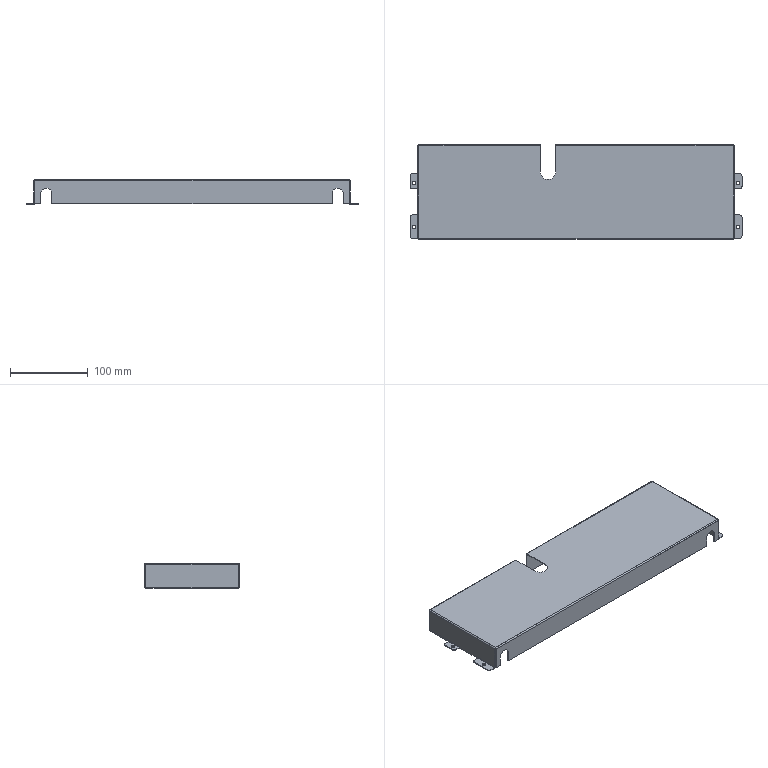Part | SolidWorks | features Cut 3, EdgeFlange 3, Fillet 1, FlatPattern 1, ICE 1, SMBaseFlange 1, SheetMetal 1 | 1 solid | 110 faces | box 427 x 122 x 32 mm | volume 79185 mm3 | plane 73 | cylinder 37 | commonest cylinder face diameters 1 x9 4.5 x8 6 x8 3 x7 14 x4 20 x1